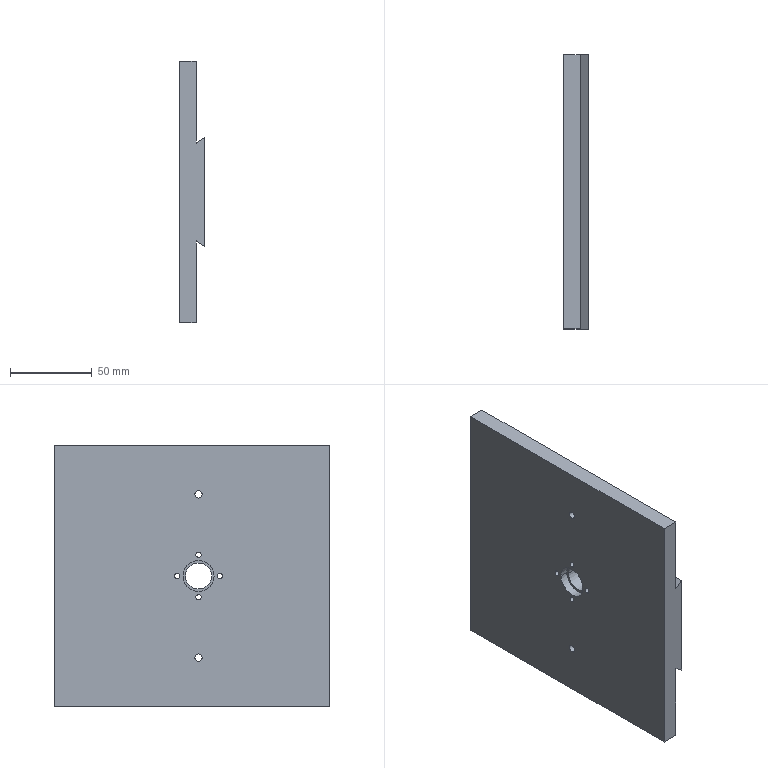Part | STEP file | 03-03 Tray support plate | 1 solid | 41 faces | box 15 x 168 x 160 mm | volume 317269 mm3 | cylinder 24 | plane 13 | cone 4 | commonest cylinder face diameters 3.3 x8 2.5 x4 4.5 x4 9 x4 16 x2 19 x2